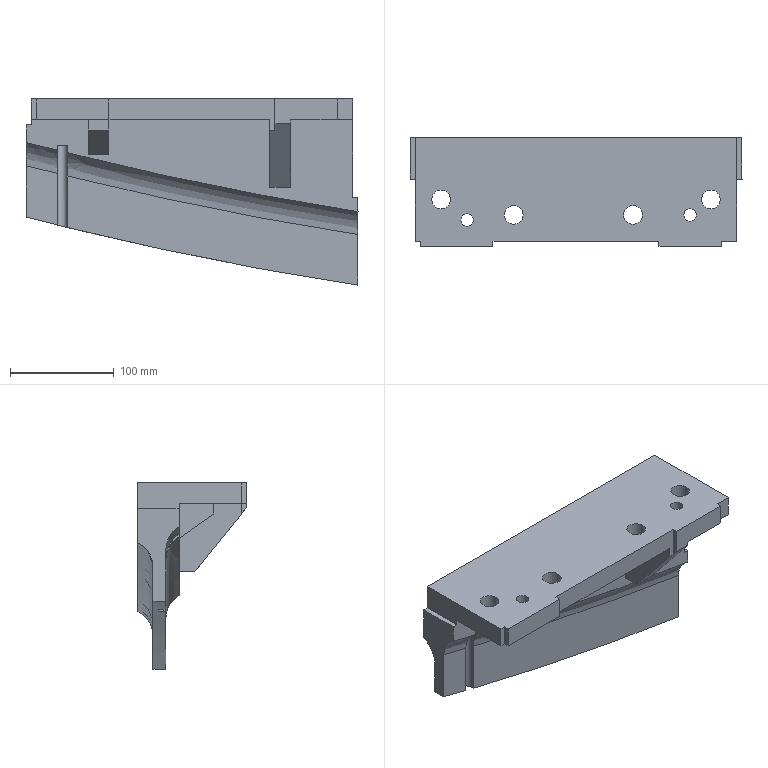Part | NX | features solid 2 | 1 solid | 53 faces | box 320 x 105 x 179.471 mm | volume 1806515 mm3 | plane 35 | cylinder 11 | spline 7 | commonest cylinder face diameters 18 x4 26 x4 12 x2 10 x1